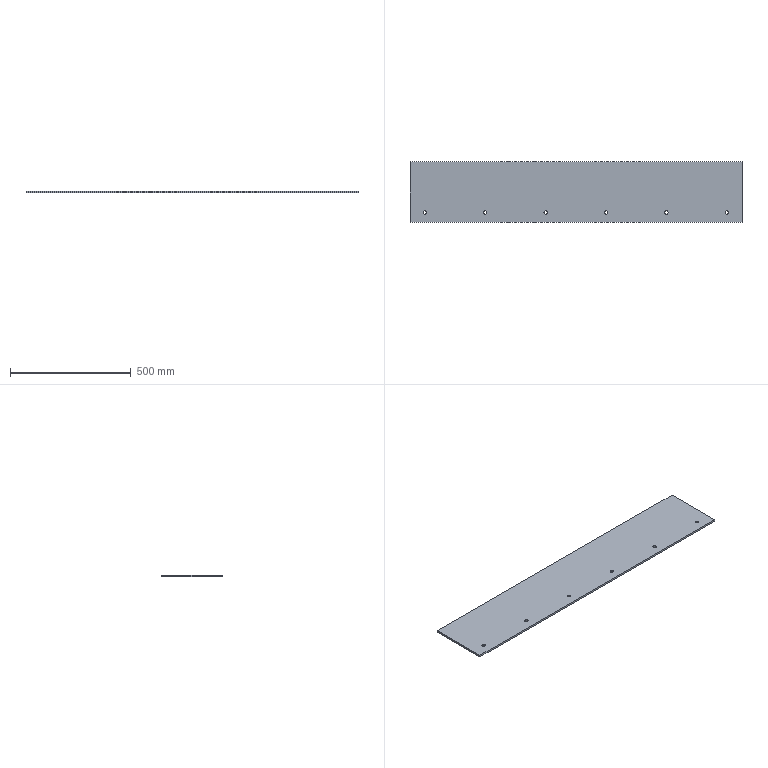Part | STEP file | Rubber plate 2_Default<As machined> | 1 solid | 18 faces | box 1374 x 250 x 8 mm | volume 2740611 mm3 | cylinder 12 | plane 6 | commonest cylinder face diameters 14 x12
STEP:
#1=CARTESIAN_POINT('',(0.,0.,0.));
#2=DIRECTION('',(0.,0.,1.));
#3=DIRECTION('',(1.,0.,0.));
#4=AXIS2_PLACEMENT_3D('',#1,#2,#3);
#5=CARTESIAN_POINT('',(-632.5,40.,8.));
#6=VERTEX_POINT('',#5);
#7=CARTESIAN_POINT('',(-632.5,40.,0.));
#8=VERTEX_POINT('',#7);
#9=CARTESIAN_POINT('',(-632.5,40.,8.));
#10=DIRECTION('',(0.,0.,-1.));
#11=VECTOR('',#10,1.);
#12=LINE('',#9,#11);
#13=CARTESIAN_POINT('',(-625.5,40.,8.));
#14=DIRECTION('',(0.,0.,-1.));
#15=DIRECTION('',(-1.,0.,0.));
#16=AXIS2_PLACEMENT_3D('',#13,#14,#15);
#17=CYLINDRICAL_SURFACE('',#16,7.);
#18=CARTESIAN_POINT('',(6.283,0.));
#19=DIRECTION('',(0.,1.));
#20=VECTOR('',#19,1.);
#21=LINE('',#18,#20);
#22=(GEOMETRIC_REPRESENTATION_CONTEXT(2)PARAMETRIC_REPRESENTATION_CONTEXT()REPRESENTATION_CONTEXT('',''));
#23=DEFINITIONAL_REPRESENTATION('',(#21),#22);
#24=PCURVE('',#17,#23);
#25=CARTESIAN_POINT('',(-625.5,40.,8.));
#26=DIRECTION('',(0.,0.,-1.));
#27=DIRECTION('',(-1.,0.,0.));
#28=AXIS2_PLACEMENT_3D('',#25,#26,#27);
#29=CYLINDRICAL_SURFACE('',#28,7.);
#30=CARTESIAN_POINT('',(0.,0.));
#31=DIRECTION('',(0.,1.));
#32=VECTOR('',#31,1.);
#33=LINE('',#30,#32);
#34=(GEOMETRIC_REPRESENTATION_CONTEXT(2)PARAMETRIC_REPRESENTATION_CONTEXT()REPRESENTATION_CONTEXT('',''));
#35=DEFINITIONAL_REPRESENTATION('',(#33),#34);
#36=PCURVE('',#29,#35);
#37=SURFACE_CURVE('',#12,(#24,#36),.PCURVE_S1.);
#38=EDGE_CURVE('',#6,#8,#37,.T.);
#39=ORIENTED_EDGE('',*,*,#38,.T.);
#40=CARTESIAN_POINT('',(-618.5,40.,0.));
#41=VERTEX_POINT('',#40);
#42=CARTESIAN_POINT('',(-625.5,40.,0.));
#43=DIRECTION('',(0.,0.,1.));
#44=DIRECTION('',(1.,0.,0.));
#45=AXIS2_PLACEMENT_3D('',#42,#43,#44);
#46=CIRCLE('',#45,7.);
#47=CARTESIAN_POINT('',(9.425,8.));
#48=DIRECTION('',(-1.,0.));
#49=VECTOR('',#48,1.);
#50=LINE('',#47,#49);
#51=(GEOMETRIC_REPRESENTATION_CONTEXT(2)PARAMETRIC_REPRESENTATION_CONTEXT()REPRESENTATION_CONTEXT('',''));
#52=DEFINITIONAL_REPRESENTATION('',(#50),#51);
#53=PCURVE('',#17,#52);
#54=CARTESIAN_POINT('',(0.,0.,0.));
#55=DIRECTION('',(0.,0.,1.));
#56=DIRECTION('',(1.,0.,0.));
#57=AXIS2_PLACEMENT_3D('',#54,#55,#56);
#58=PLANE('',#57);
#59=CARTESIAN_POINT('',(-625.5,40.));
#60=DIRECTION('',(1.,0.));
#61=AXIS2_PLACEMENT_2D('',#59,#60);
#62=CIRCLE('',#61,7.);
#63=(GEOMETRIC_REPRESENTATION_CONTEXT(2)PARAMETRIC_REPRESENTATION_CONTEXT()REPRESENTATION_CONTEXT('',''));
#64=DEFINITIONAL_REPRESENTATION('',(#62),#63);
#65=PCURVE('',#58,#64);
#66=SURFACE_CURVE('',#46,(#53,#65),.PCURVE_S1.);
#67=EDGE_CURVE('',#8,#41,#66,.T.);
#68=ORIENTED_EDGE('',*,*,#67,.T.);
#69=CARTESIAN_POINT('',(-618.5,40.,8.));
#70=VERTEX_POINT('',#69);
#71=CARTESIAN_POINT('',(-618.5,40.,8.));
#72=DIRECTION('',(0.,0.,-1.));
#73=VECTOR('',#72,1.);
#74=LINE('',#71,#73);
#75=CARTESIAN_POINT('',(3.142,0.));
#76=DIRECTION('',(0.,1.));
#77=VECTOR('',#76,1.);
#78=LINE('',#75,#77);
#79=(GEOMETRIC_REPRESENTATION_CONTEXT(2)PARAMETRIC_REPRESENTATION_CONTEXT()REPRESENTATION_CONTEXT('',''));
#80=DEFINITIONAL_REPRESENTATION('',(#78),#79);
#81=PCURVE('',#17,#80);
#82=CARTESIAN_POINT('',(3.142,0.));
#83=DIRECTION('',(0.,1.));
#84=VECTOR('',#83,1.);
#85=LINE('',#82,#84);
#86=(GEOMETRIC_REPRESENTATION_CONTEXT(2)PARAMETRIC_REPRESENTATION_CONTEXT()REPRESENTATION_CONTEXT('',''));
#87=DEFINITIONAL_REPRESENTATION('',(#85),#86);
#88=PCURVE('',#29,#87);
#89=SURFACE_CURVE('',#74,(#81,#88),.PCURVE_S1.);
#90=EDGE_CURVE('',#70,#41,#89,.T.);
#91=ORIENTED_EDGE('',*,*,#90,.F.);
#92=CARTESIAN_POINT('',(-625.5,40.,8.));
#93=DIRECTION('',(0.,0.,1.));
#94=DIRECTION('',(1.,0.,0.));
#95=AXIS2_PLACEMENT_3D('',#92,#93,#94);
#96=CIRCLE('',#95,7.);
#97=CARTESIAN_POINT('',(9.425,0.));
#98=DIRECTION('',(-1.,0.));
#99=VECTOR('',#98,1.);
#100=LINE('',#97,#99);
#101=(GEOMETRIC_REPRESENTATION_CONTEXT(2)PARAMETRIC_REPRESENTATION_CONTEXT()REPRESENTATION_CONTEXT('',''));
#102=DEFINITIONAL_REPRESENTATION('',(#100),#101);
#103=PCURVE('',#17,#102);
#104=CARTESIAN_POINT('',(0.,0.,8.));
#105=DIRECTION('',(0.,0.,1.));
#106=DIRECTION('',(1.,0.,0.));
#107=AXIS2_PLACEMENT_3D('',#104,#105,#106);
#108=PLANE('',#107);
#109=CARTESIAN_POINT('',(-625.5,40.));
#110=DIRECTION('',(1.,0.));
#111=AXIS2_PLACEMENT_2D('',#109,#110);
#112=CIRCLE('',#111,7.);
#113=(GEOMETRIC_REPRESENTATION_CONTEXT(2)PARAMETRIC_REPRESENTATION_CONTEXT()REPRESENTATION_CONTEXT('',''));
#114=DEFINITIONAL_REPRESENTATION('',(#112),#113);
#115=PCURVE('',#108,#114);
#116=SURFACE_CURVE('',#96,(#103,#115),.PCURVE_S1.);
#117=EDGE_CURVE('',#6,#70,#116,.T.);
#118=ORIENTED_EDGE('',*,*,#117,.F.);
#119=EDGE_LOOP('',(#39,#68,#91,#118));
#120=FACE_BOUND('',#119,.F.);
#121=ADVANCED_FACE('',(#120),#17,.F.);
#122=CARTESIAN_POINT('',(-382.5,40.,8.));
#123=VERTEX_POINT('',#122);
#124=CARTESIAN_POINT('',(-382.5,40.,0.));
#125=VERTEX_POINT('',#124);
#126=CARTESIAN_POINT('',(-382.5,40.,8.));
#127=DIRECTION('',(0.,0.,-1.));
#128=VECTOR('',#127,1.);
#129=LINE('',#126,#128);
#130=CARTESIAN_POINT('',(-375.5,40.,8.));
#131=DIRECTION('',(0.,0.,-1.));
#132=DIRECTION('',(-1.,0.,0.));
#133=AXIS2_PLACEMENT_3D('',#130,#131,#132);
#134=CYLINDRICAL_SURFACE('',#133,7.);
#135=CARTESIAN_POINT('',(6.283,0.));
#136=DIRECTION('',(0.,1.));
#137=VECTOR('',#136,1.);
#138=LINE('',#135,#137);
#139=(GEOMETRIC_REPRESENTATION_CONTEXT(2)PARAMETRIC_REPRESENTATION_CONTEXT()REPRESENTATION_CONTEXT('',''));
#140=DEFINITIONAL_REPRESENTATION('',(#138),#139);
#141=PCURVE('',#134,#140);
#142=CARTESIAN_POINT('',(-375.5,40.,8.));
#143=DIRECTION('',(0.,0.,-1.));
#144=DIRECTION('',(-1.,0.,0.));
#145=AXIS2_PLACEMENT_3D('',#142,#143,#144);
#146=CYLINDRICAL_SURFACE('',#145,7.);
#147=CARTESIAN_POINT('',(0.,0.));
#148=DIRECTION('',(0.,1.));
#149=VECTOR('',#148,1.);
#150=LINE('',#147,#149);
#151=(GEOMETRIC_REPRESENTATION_CONTEXT(2)PARAMETRIC_REPRESENTATION_CONTEXT()REPRESENTATION_CONTEXT('',''));
#152=DEFINITIONAL_REPRESENTATION('',(#150),#151);
#153=PCURVE('',#146,#152);
#154=SURFACE_CURVE('',#129,(#141,#153),.PCURVE_S1.);
#155=EDGE_CURVE('',#123,#125,#154,.T.);
#156=ORIENTED_EDGE('',*,*,#155,.T.);
#157=CARTESIAN_POINT('',(-368.5,40.,0.));
#158=VERTEX_POINT('',#157);
#159=CARTESIAN_POINT('',(-375.5,40.,0.));
#160=DIRECTION('',(0.,0.,1.));
#161=DIRECTION('',(1.,0.,0.));
#162=AXIS2_PLACEMENT_3D('',#159,#160,#161);
#163=CIRCLE('',#162,7.);
#164=CARTESIAN_POINT('',(9.425,8.));
#165=DIRECTION('',(-1.,0.));
#166=VECTOR('',#165,1.);
#167=LINE('',#164,#166);
#168=(GEOMETRIC_REPRESENTATION_CONTEXT(2)PARAMETRIC_REPRESENTATION_CONTEXT()REPRESENTATION_CONTEXT('',''));
#169=DEFINITIONAL_REPRESENTATION('',(#167),#168);
#170=PCURVE('',#134,#169);
#171=CARTESIAN_POINT('',(-375.5,40.));
#172=DIRECTION('',(1.,0.));
#173=AXIS2_PLACEMENT_2D('',#171,#172);
#174=CIRCLE('',#173,7.);
#175=(GEOMETRIC_REPRESENTATION_CONTEXT(2)PARAMETRIC_REPRESENTATION_CONTEXT()REPRESENTATION_CONTEXT('',''));
#176=DEFINITIONAL_REPRESENTATION('',(#174),#175);
#177=PCURVE('',#58,#176);
#178=SURFACE_CURVE('',#163,(#170,#177),.PCURVE_S1.);
#179=EDGE_CURVE('',#125,#158,#178,.T.);
#180=ORIENTED_EDGE('',*,*,#179,.T.);
#181=CARTESIAN_POINT('',(-368.5,40.,8.));
#182=VERTEX_POINT('',#181);
#183=CARTESIAN_POINT('',(-368.5,40.,8.));
#184=DIRECTION('',(0.,0.,-1.));
#185=VECTOR('',#184,1.);
#186=LINE('',#183,#185);
#187=CARTESIAN_POINT('',(3.142,0.));
#188=DIRECTION('',(0.,1.));
#189=VECTOR('',#188,1.);
#190=LINE('',#187,#189);
#191=(GEOMETRIC_REPRESENTATION_CONTEXT(2)PARAMETRIC_REPRESENTATION_CONTEXT()REPRESENTATION_CONTEXT('',''));
#192=DEFINITIONAL_REPRESENTATION('',(#190),#191);
#193=PCURVE('',#134,#192);
#194=CARTESIAN_POINT('',(3.142,0.));
#195=DIRECTION('',(0.,1.));
#196=VECTOR('',#195,1.);
#197=LINE('',#194,#196);
#198=(GEOMETRIC_REPRESENTATION_CONTEXT(2)PARAMETRIC_REPRESENTATION_CONTEXT()REPRESENTATION_CONTEXT('',''));
#199=DEFINITIONAL_REPRESENTATION('',(#197),#198);
#200=PCURVE('',#146,#199);
#201=SURFACE_CURVE('',#186,(#193,#200),.PCURVE_S1.);
#202=EDGE_CURVE('',#182,#158,#201,.T.);
#203=ORIENTED_EDGE('',*,*,#202,.F.);
#204=CARTESIAN_POINT('',(-375.5,40.,8.));
#205=DIRECTION('',(0.,0.,1.));
#206=DIRECTION('',(1.,0.,0.));
#207=AXIS2_PLACEMENT_3D('',#204,#205,#206);
#208=CIRCLE('',#207,7.);
#209=CARTESIAN_POINT('',(9.425,0.));
#210=DIRECTION('',(-1.,0.));
#211=VECTOR('',#210,1.);
#212=LINE('',#209,#211);
#213=(GEOMETRIC_REPRESENTATION_CONTEXT(2)PARAMETRIC_REPRESENTATION_CONTEXT()REPRESENTATION_CONTEXT('',''));
#214=DEFINITIONAL_REPRESENTATION('',(#212),#213);
#215=PCURVE('',#134,#214);
#216=CARTESIAN_POINT('',(-375.5,40.));
#217=DIRECTION('',(1.,0.));
#218=AXIS2_PLACEMENT_2D('',#216,#217);
#219=CIRCLE('',#218,7.);
#220=(GEOMETRIC_REPRESENTATION_CONTEXT(2)PARAMETRIC_REPRESENTATION_CONTEXT()REPRESENTATION_CONTEXT('',''));
#221=DEFINITIONAL_REPRESENTATION('',(#219),#220);
#222=PCURVE('',#108,#221);
#223=SURFACE_CURVE('',#208,(#215,#222),.PCURVE_S1.);
#224=EDGE_CURVE('',#123,#182,#223,.T.);
#225=ORIENTED_EDGE('',*,*,#224,.F.);
#226=EDGE_LOOP('',(#156,#180,#203,#225));
#227=FACE_BOUND('',#226,.F.);
#228=ADVANCED_FACE('',(#227),#134,.F.);
#229=CARTESIAN_POINT('',(-132.5,40.,8.));
#230=VERTEX_POINT('',#229);
#231=CARTESIAN_POINT('',(-132.5,40.,0.));
#232=VERTEX_POINT('',#231);
#233=CARTESIAN_POINT('',(-132.5,40.,8.));
#234=DIRECTION('',(0.,0.,-1.));
#235=VECTOR('',#234,1.);
#236=LINE('',#233,#235);
#237=CARTESIAN_POINT('',(-125.5,40.,8.));
#238=DIRECTION('',(0.,0.,-1.));
#239=DIRECTION('',(-1.,0.,0.));
#240=AXIS2_PLACEMENT_3D('',#237,#238,#239);
#241=CYLINDRICAL_SURFACE('',#240,7.);
#242=CARTESIAN_POINT('',(6.283,0.));
#243=DIRECTION('',(0.,1.));
#244=VECTOR('',#243,1.);
#245=LINE('',#242,#244);
#246=(GEOMETRIC_REPRESENTATION_CONTEXT(2)PARAMETRIC_REPRESENTATION_CONTEXT()REPRESENTATION_CONTEXT('',''));
#247=DEFINITIONAL_REPRESENTATION('',(#245),#246);
#248=PCURVE('',#241,#247);
#249=CARTESIAN_POINT('',(-125.5,40.,8.));
#250=DIRECTION('',(0.,0.,-1.));
#251=DIRECTION('',(-1.,0.,0.));
#252=AXIS2_PLACEMENT_3D('',#249,#250,#251);
#253=CYLINDRICAL_SURFACE('',#252,7.);
#254=CARTESIAN_POINT('',(0.,0.));
#255=DIRECTION('',(0.,1.));
#256=VECTOR('',#255,1.);
#257=LINE('',#254,#256);
#258=(GEOMETRIC_REPRESENTATION_CONTEXT(2)PARAMETRIC_REPRESENTATION_CONTEXT()REPRESENTATION_CONTEXT('',''));
#259=DEFINITIONAL_REPRESENTATION('',(#257),#258);
#260=PCURVE('',#253,#259);
#261=SURFACE_CURVE('',#236,(#248,#260),.PCURVE_S1.);
#262=EDGE_CURVE('',#230,#232,#261,.T.);
#263=ORIENTED_EDGE('',*,*,#262,.T.);
#264=CARTESIAN_POINT('',(-118.5,40.,0.));
#265=VERTEX_POINT('',#264);
#266=CARTESIAN_POINT('',(-125.5,40.,0.));
#267=DIRECTION('',(0.,0.,1.));
#268=DIRECTION('',(1.,0.,0.));
#269=AXIS2_PLACEMENT_3D('',#266,#267,#268);
#270=CIRCLE('',#269,7.);
#271=CARTESIAN_POINT('',(9.425,8.));
#272=DIRECTION('',(-1.,0.));
#273=VECTOR('',#272,1.);
#274=LINE('',#271,#273);
#275=(GEOMETRIC_REPRESENTATION_CONTEXT(2)PARAMETRIC_REPRESENTATION_CONTEXT()REPRESENTATION_CONTEXT('',''));
#276=DEFINITIONAL_REPRESENTATION('',(#274),#275);
#277=PCURVE('',#241,#276);
#278=CARTESIAN_POINT('',(-125.5,40.));
#279=DIRECTION('',(1.,0.));
#280=AXIS2_PLACEMENT_2D('',#278,#279);
#281=CIRCLE('',#280,7.);
#282=(GEOMETRIC_REPRESENTATION_CONTEXT(2)PARAMETRIC_REPRESENTATION_CONTEXT()REPRESENTATION_CONTEXT('',''));
#283=DEFINITIONAL_REPRESENTATION('',(#281),#282);
#284=PCURVE('',#58,#283);
#285=SURFACE_CURVE('',#270,(#277,#284),.PCURVE_S1.);
#286=EDGE_CURVE('',#232,#265,#285,.T.);
#287=ORIENTED_EDGE('',*,*,#286,.T.);
#288=CARTESIAN_POINT('',(-118.5,40.,8.));
#289=VERTEX_POINT('',#288);
#290=CARTESIAN_POINT('',(-118.5,40.,8.));
#291=DIRECTION('',(0.,0.,-1.));
#292=VECTOR('',#291,1.);
#293=LINE('',#290,#292);
#294=CARTESIAN_POINT('',(3.142,0.));
#295=DIRECTION('',(0.,1.));
#296=VECTOR('',#295,1.);
#297=LINE('',#294,#296);
#298=(GEOMETRIC_REPRESENTATION_CONTEXT(2)PARAMETRIC_REPRESENTATION_CONTEXT()REPRESENTATION_CONTEXT('',''));
#299=DEFINITIONAL_REPRESENTATION('',(#297),#298);
#300=PCURVE('',#241,#299);
#301=CARTESIAN_POINT('',(3.142,0.));
#302=DIRECTION('',(0.,1.));
#303=VECTOR('',#302,1.);
#304=LINE('',#301,#303);
#305=(GEOMETRIC_REPRESENTATION_CONTEXT(2)PARAMETRIC_REPRESENTATION_CONTEXT()REPRESENTATION_CONTEXT('',''));
#306=DEFINITIONAL_REPRESENTATION('',(#304),#305);
#307=PCURVE('',#253,#306);
#308=SURFACE_CURVE('',#293,(#300,#307),.PCURVE_S1.);
#309=EDGE_CURVE('',#289,#265,#308,.T.);
#310=ORIENTED_EDGE('',*,*,#309,.F.);
#311=CARTESIAN_POINT('',(-125.5,40.,8.));
#312=DIRECTION('',(0.,0.,1.));
#313=DIRECTION('',(1.,0.,0.));
#314=AXIS2_PLACEMENT_3D('',#311,#312,#313);
#315=CIRCLE('',#314,7.);
#316=CARTESIAN_POINT('',(9.425,0.));
#317=DIRECTION('',(-1.,0.));
#318=VECTOR('',#317,1.);
#319=LINE('',#316,#318);
#320=(GEOMETRIC_REPRESENTATION_CONTEXT(2)PARAMETRIC_REPRESENTATION_CONTEXT()REPRESENTATION_CONTEXT('',''));
#321=DEFINITIONAL_REPRESENTATION('',(#319),#320);
#322=PCURVE('',#241,#321);
#323=CARTESIAN_POINT('',(-125.5,40.));
#324=DIRECTION('',(1.,0.));
#325=AXIS2_PLACEMENT_2D('',#323,#324);
#326=CIRCLE('',#325,7.);
#327=(GEOMETRIC_REPRESENTATION_CONTEXT(2)PARAMETRIC_REPRESENTATION_CONTEXT()REPRESENTATION_CONTEXT('',''));
#328=DEFINITIONAL_REPRESENTATION('',(#326),#327);
#329=PCURVE('',#108,#328);
#330=SURFACE_CURVE('',#315,(#322,#329),.PCURVE_S1.);
#331=EDGE_CURVE('',#230,#289,#330,.T.);
#332=ORIENTED_EDGE('',*,*,#331,.F.);
#333=EDGE_LOOP('',(#263,#287,#310,#332));
#334=FACE_BOUND('',#333,.F.);
#335=ADVANCED_FACE('',(#334),#241,.F.);
#336=CARTESIAN_POINT('',(117.5,40.,8.));
#337=VERTEX_POINT('',#336);
#338=CARTESIAN_POINT('',(117.5,40.,0.));
#339=VERTEX_POINT('',#338);
#340=CARTESIAN_POINT('',(117.5,40.,8.));
#341=DIRECTION('',(0.,0.,-1.));
#342=VECTOR('',#341,1.);
#343=LINE('',#340,#342);
#344=CARTESIAN_POINT('',(124.5,40.,8.));
#345=DIRECTION('',(0.,0.,-1.));
#346=DIRECTION('',(-1.,0.,0.));
#347=AXIS2_PLACEMENT_3D('',#344,#345,#346);
#348=CYLINDRICAL_SURFACE('',#347,7.);
#349=CARTESIAN_POINT('',(6.283,0.));
#350=DIRECTION('',(0.,1.));
#351=VECTOR('',#350,1.);
#352=LINE('',#349,#351);
#353=(GEOMETRIC_REPRESENTATION_CONTEXT(2)PARAMETRIC_REPRESENTATION_CONTEXT()REPRESENTATION_CONTEXT('',''));
#354=DEFINITIONAL_REPRESENTATION('',(#352),#353);
#355=PCURVE('',#348,#354);
#356=CARTESIAN_POINT('',(124.5,40.,8.));
#357=DIRECTION('',(0.,0.,-1.));
#358=DIRECTION('',(-1.,0.,0.));
#359=AXIS2_PLACEMENT_3D('',#356,#357,#358);
#360=CYLINDRICAL_SURFACE('',#359,7.);
#361=CARTESIAN_POINT('',(0.,0.));
#362=DIRECTION('',(0.,1.));
#363=VECTOR('',#362,1.);
#364=LINE('',#361,#363);
#365=(GEOMETRIC_REPRESENTATION_CONTEXT(2)PARAMETRIC_REPRESENTATION_CONTEXT()REPRESENTATION_CONTEXT('',''));
#366=DEFINITIONAL_REPRESENTATION('',(#364),#365);
#367=PCURVE('',#360,#366);
#368=SURFACE_CURVE('',#343,(#355,#367),.PCURVE_S1.);
#369=EDGE_CURVE('',#337,#339,#368,.T.);
#370=ORIENTED_EDGE('',*,*,#369,.T.);
#371=CARTESIAN_POINT('',(131.5,40.,0.));
#372=VERTEX_POINT('',#371);
#373=CARTESIAN_POINT('',(124.5,40.,0.));
#374=DIRECTION('',(0.,0.,1.));
#375=DIRECTION('',(1.,0.,0.));
#376=AXIS2_PLACEMENT_3D('',#373,#374,#375);
#377=CIRCLE('',#376,7.);
#378=CARTESIAN_POINT('',(9.425,8.));
#379=DIRECTION('',(-1.,0.));
#380=VECTOR('',#379,1.);
#381=LINE('',#378,#380);
#382=(GEOMETRIC_REPRESENTATION_CONTEXT(2)PARAMETRIC_REPRESENTATION_CONTEXT()REPRESENTATION_CONTEXT('',''));
#383=DEFINITIONAL_REPRESENTATION('',(#381),#382);
#384=PCURVE('',#348,#383);
#385=CARTESIAN_POINT('',(124.5,40.));
#386=DIRECTION('',(1.,0.));
#387=AXIS2_PLACEMENT_2D('',#385,#386);
#388=CIRCLE('',#387,7.);
#389=(GEOMETRIC_REPRESENTATION_CONTEXT(2)PARAMETRIC_REPRESENTATION_CONTEXT()REPRESENTATION_CONTEXT('',''));
#390=DEFINITIONAL_REPRESENTATION('',(#388),#389);
#391=PCURVE('',#58,#390);
#392=SURFACE_CURVE('',#377,(#384,#391),.PCURVE_S1.);
#393=EDGE_CURVE('',#339,#372,#392,.T.);
#394=ORIENTED_EDGE('',*,*,#393,.T.);
#395=CARTESIAN_POINT('',(131.5,40.,8.));
#396=VERTEX_POINT('',#395);
#397=CARTESIAN_POINT('',(131.5,40.,8.));
#398=DIRECTION('',(0.,0.,-1.));
#399=VECTOR('',#398,1.);
#400=LINE('',#397,#399);
#401=CARTESIAN_POINT('',(3.142,0.));
#402=DIRECTION('',(0.,1.));
#403=VECTOR('',#402,1.);
#404=LINE('',#401,#403);
#405=(GEOMETRIC_REPRESENTATION_CONTEXT(2)PARAMETRIC_REPRESENTATION_CONTEXT()REPRESENTATION_CONTEXT('',''));
#406=DEFINITIONAL_REPRESENTATION('',(#404),#405);
#407=PCURVE('',#348,#406);
#408=CARTESIAN_POINT('',(3.142,0.));
#409=DIRECTION('',(0.,1.));
#410=VECTOR('',#409,1.);
#411=LINE('',#408,#410);
#412=(GEOMETRIC_REPRESENTATION_CONTEXT(2)PARAMETRIC_REPRESENTATION_CONTEXT()REPRESENTATION_CONTEXT('',''));
#413=DEFINITIONAL_REPRESENTATION('',(#411),#412);
#414=PCURVE('',#360,#413);
#415=SURFACE_CURVE('',#400,(#407,#414),.PCURVE_S1.);
#416=EDGE_CURVE('',#396,#372,#415,.T.);
#417=ORIENTED_EDGE('',*,*,#416,.F.);
#418=CARTESIAN_POINT('',(124.5,40.,8.));
#419=DIRECTION('',(0.,0.,1.));
#420=DIRECTION('',(1.,0.,0.));
#421=AXIS2_PLACEMENT_3D('',#418,#419,#420);
#422=CIRCLE('',#421,7.);
#423=CARTESIAN_POINT('',(9.425,0.));
#424=DIRECTION('',(-1.,0.));
#425=VECTOR('',#424,1.);
#426=LINE('',#423,#425);
#427=(GEOMETRIC_REPRESENTATION_CONTEXT(2)PARAMETRIC_REPRESENTATION_CONTEXT()REPRESENTATION_CONTEXT('',''));
#428=DEFINITIONAL_REPRESENTATION('',(#426),#427);
#429=PCURVE('',#348,#428);
#430=CARTESIAN_POINT('',(124.5,40.));
#431=DIRECTION('',(1.,0.));
#432=AXIS2_PLACEMENT_2D('',#430,#431);
#433=CIRCLE('',#432,7.);
#434=(GEOMETRIC_REPRESENTATION_CONTEXT(2)PARAMETRIC_REPRESENTATION_CONTEXT()REPRESENTATION_CONTEXT('',''));
#435=DEFINITIONAL_REPRESENTATION('',(#433),#434);
#436=PCURVE('',#108,#435);
#437=SURFACE_CURVE('',#422,(#429,#436),.PCURVE_S1.);
#438=EDGE_CURVE('',#337,#396,#437,.T.);
#439=ORIENTED_EDGE('',*,*,#438,.F.);
#440=EDGE_LOOP('',(#370,#394,#417,#439));
#441=FACE_BOUND('',#440,.F.);
#442=ADVANCED_FACE('',(#441),#348,.F.);
#443=CARTESIAN_POINT('',(367.5,40.,8.));
#444=VERTEX_POINT('',#443);
#445=CARTESIAN_POINT('',(367.5,40.,0.));
#446=VERTEX_POINT('',#445);
#447=CARTESIAN_POINT('',(367.5,40.,8.));
#448=DIRECTION('',(0.,0.,-1.));
#449=VECTOR('',#448,1.);
#450=LINE('',#447,#449);
#451=CARTESIAN_POINT('',(374.5,40.,8.));
#452=DIRECTION('',(0.,0.,-1.));
#453=DIRECTION('',(-1.,0.,0.));
#454=AXIS2_PLACEMENT_3D('',#451,#452,#453);
#455=CYLINDRICAL_SURFACE('',#454,7.);
#456=CARTESIAN_POINT('',(6.283,0.));
#457=DIRECTION('',(0.,1.));
#458=VECTOR('',#457,1.);
#459=LINE('',#456,#458);
#460=(GEOMETRIC_REPRESENTATION_CONTEXT(2)PARAMETRIC_REPRESENTATION_CONTEXT()REPRESENTATION_CONTEXT('',''));
#461=DEFINITIONAL_REPRESENTATION('',(#459),#460);
#462=PCURVE('',#455,#461);
#463=CARTESIAN_POINT('',(374.5,40.,8.));
#464=DIRECTION('',(0.,0.,-1.));
#465=DIRECTION('',(-1.,0.,0.));
#466=AXIS2_PLACEMENT_3D('',#463,#464,#465);
#467=CYLINDRICAL_SURFACE('',#466,7.);
#468=CARTESIAN_POINT('',(0.,0.));
#469=DIRECTION('',(0.,1.));
#470=VECTOR('',#469,1.);
#471=LINE('',#468,#470);
#472=(GEOMETRIC_REPRESENTATION_CONTEXT(2)PARAMETRIC_REPRESENTATION_CONTEXT()REPRESENTATION_CONTEXT('',''));
#473=DEFINITIONAL_REPRESENTATION('',(#471),#472);
#474=PCURVE('',#467,#473);
#475=SURFACE_CURVE('',#450,(#462,#474),.PCURVE_S1.);
#476=EDGE_CURVE('',#444,#446,#475,.T.);
#477=ORIENTED_EDGE('',*,*,#476,.T.);
#478=CARTESIAN_POINT('',(381.5,40.,0.));
#479=VERTEX_POINT('',#478);
#480=CARTESIAN_POINT('',(374.5,40.,0.));
#481=DIRECTION('',(0.,0.,1.));
#482=DIRECTION('',(1.,0.,0.));
#483=AXIS2_PLACEMENT_3D('',#480,#481,#482);
#484=CIRCLE('',#483,7.);
#485=CARTESIAN_POINT('',(9.425,8.));
#486=DIRECTION('',(-1.,0.));
#487=VECTOR('',#486,1.);
#488=LINE('',#485,#487);
#489=(GEOMETRIC_REPRESENTATION_CONTEXT(2)PARAMETRIC_REPRESENTATION_CONTEXT()REPRESENTATION_CONTEXT('',''));
#490=DEFINITIONAL_REPRESENTATION('',(#488),#489);
#491=PCURVE('',#455,#490);
#492=CARTESIAN_POINT('',(374.5,40.));
#493=DIRECTION('',(1.,0.));
#494=AXIS2_PLACEMENT_2D('',#492,#493);
#495=CIRCLE('',#494,7.);
#496=(GEOMETRIC_REPRESENTATION_CONTEXT(2)PARAMETRIC_REPRESENTATION_CONTEXT()REPRESENTATION_CONTEXT('',''));
#497=DEFINITIONAL_REPRESENTATION('',(#495),#496);
#498=PCURVE('',#58,#497);
#499=SURFACE_CURVE('',#484,(#491,#498),.PCURVE_S1.);
#500=EDGE_CURVE('',#446,#479,#499,.T.);
#501=ORIENTED_EDGE('',*,*,#500,.T.);
#502=CARTESIAN_POINT('',(381.5,40.,8.));
#503=VERTEX_POINT('',#502);
#504=CARTESIAN_POINT('',(381.5,40.,8.));
#505=DIRECTION('',(0.,0.,-1.));
#506=VECTOR('',#505,1.);
#507=LINE('',#504,#506);
#508=CARTESIAN_POINT('',(3.142,0.));
#509=DIRECTION('',(0.,1.));
#510=VECTOR('',#509,1.);
#511=LINE('',#508,#510);
#512=(GEOMETRIC_REPRESENTATION_CONTEXT(2)PARAMETRIC_REPRESENTATION_CONTEXT()REPRESENTATION_CONTEXT('',''));
#513=DEFINITIONAL_REPRESENTATION('',(#511),#512);
#514=PCURVE('',#455,#513);
#515=CARTESIAN_POINT('',(3.142,0.));
#516=DIRECTION('',(0.,1.));
#517=VECTOR('',#516,1.);
#518=LINE('',#515,#517);
#519=(GEOMETRIC_REPRESENTATION_CONTEXT(2)PARAMETRIC_REPRESENTATION_CONTEXT()REPRESENTATION_CONTEXT('',''));
#520=DEFINITIONAL_REPRESENTATION('',(#518),#519);
#521=PCURVE('',#467,#520);
#522=SURFACE_CURVE('',#507,(#514,#521),.PCURVE_S1.);
#523=EDGE_CURVE('',#503,#479,#522,.T.);
#524=ORIENTED_EDGE('',*,*,#523,.F.);
#525=CARTESIAN_POINT('',(374.5,40.,8.));
#526=DIRECTION('',(0.,0.,1.));
#527=DIRECTION('',(1.,0.,0.));
#528=AXIS2_PLACEMENT_3D('',#525,#526,#527);
#529=CIRCLE('',#528,7.);
#530=CARTESIAN_POINT('',(9.425,0.));
#531=DIRECTION('',(-1.,0.));
#532=VECTOR('',#531,1.);
#533=LINE('',#530,#532);
#534=(GEOMETRIC_REPRESENTATION_CONTEXT(2)PARAMETRIC_REPRESENTATION_CONTEXT()REPRESENTATION_CONTEXT('',''));
#535=DEFINITIONAL_REPRESENTATION('',(#533),#534);
#536=PCURVE('',#455,#535);
#537=CARTESIAN_POINT('',(374.5,40.));
#538=DIRECTION('',(1.,0.));
#539=AXIS2_PLACEMENT_2D('',#537,#538);
#540=CIRCLE('',#539,7.);
#541=(GEOMETRIC_REPRESENTATION_CONTEXT(2)PARAMETRIC_REPRESENTATION_CONTEXT()REPRESENTATION_CONTEXT('',''));
#542=DEFINITIONAL_REPRESENTATION('',(#540),#541);
#543=PCURVE('',#108,#542);
#544=SURFACE_CURVE('',#529,(#536,#543),.PCURVE_S1.);
#545=EDGE_CURVE('',#444,#503,#544,.T.);
#546=ORIENTED_EDGE('',*,*,#545,.F.);
#547=EDGE_LOOP('',(#477,#501,#524,#546));
#548=FACE_BOUND('',#547,.F.);
#549=ADVANCED_FACE('',(#548),#455,.F.);
#550=CARTESIAN_POINT('',(617.5,40.,8.));
#551=VERTEX_POINT('',#550);
#552=CARTESIAN_POINT('',(617.5,40.,0.));
#553=VERTEX_POINT('',#552);
#554=CARTESIAN_POINT('',(617.5,40.,8.));
#555=DIRECTION('',(0.,0.,-1.));
#556=VECTOR('',#555,1.);
#557=LINE('',#554,#556);
#558=CARTESIAN_POINT('',(624.5,40.,8.));
#559=DIRECTION('',(0.,0.,-1.));
#560=DIRECTION('',(-1.,0.,0.));
#561=AXIS2_PLACEMENT_3D('',#558,#559,#560);
#562=CYLINDRICAL_SURFACE('',#561,7.);
#563=CARTESIAN_POINT('',(6.283,0.));
#564=DIRECTION('',(0.,1.));
#565=VECTOR('',#564,1.);
#566=LINE('',#563,#565);
#567=(GEOMETRIC_REPRESENTATION_CONTEXT(2)PARAMETRIC_REPRESENTATION_CONTEXT()REPRESENTATION_CONTEXT('',''));
#568=DEFINITIONAL_REPRESENTATION('',(#566),#567);
#569=PCURVE('',#562,#568);
#570=CARTESIAN_POINT('',(624.5,40.,8.));
#571=DIRECTION('',(0.,0.,-1.));
#572=DIRECTION('',(-1.,0.,0.));
#573=AXIS2_PLACEMENT_3D('',#570,#571,#572);
#574=CYLINDRICAL_SURFACE('',#573,7.);
#575=CARTESIAN_POINT('',(0.,0.));
#576=DIRECTION('',(0.,1.));
#577=VECTOR('',#576,1.);
#578=LINE('',#575,#577);
#579=(GEOMETRIC_REPRESENTATION_CONTEXT(2)PARAMETRIC_REPRESENTATION_CONTEXT()REPRESENTATION_CONTEXT('',''));
#580=DEFINITIONAL_REPRESENTATION('',(#578),#579);
#581=PCURVE('',#574,#580);
#582=SURFACE_CURVE('',#557,(#569,#581),.PCURVE_S1.);
#583=EDGE_CURVE('',#551,#553,#582,.T.);
#584=ORIENTED_EDGE('',*,*,#583,.T.);
#585=CARTESIAN_POINT('',(631.5,40.,0.));
#586=VERTEX_POINT('',#585);
#587=CARTESIAN_POINT('',(624.5,40.,0.));
#588=DIRECTION('',(0.,0.,1.));
#589=DIRECTION('',(1.,0.,0.));
#590=AXIS2_PLACEMENT_3D('',#587,#588,#589);
#591=CIRCLE('',#590,7.);
#592=CARTESIAN_POINT('',(9.425,8.));
#593=DIRECTION('',(-1.,0.));
#594=VECTOR('',#593,1.);
#595=LINE('',#592,#594);
#596=(GEOMETRIC_REPRESENTATION_CONTEXT(2)PARAMETRIC_REPRESENTATION_CONTEXT()REPRESENTATION_CONTEXT('',''));
#597=DEFINITIONAL_REPRESENTATION('',(#595),#596);
#598=PCURVE('',#562,#597);
#599=CARTESIAN_POINT('',(624.5,40.));
#600=DIRECTION('',(1.,0.));
#601=AXIS2_PLACEMENT_2D('',#599,#600);
#602=CIRCLE('',#601,7.);
#603=(GEOMETRIC_REPRESENTATION_CONTEXT(2)PARAMETRIC_REPRESENTATION_CONTEXT()REPRESENTATION_CONTEXT('',''));
#604=DEFINITIONAL_REPRESENTATION('',(#602),#603);
#605=PCURVE('',#58,#604);
#606=SURFACE_CURVE('',#591,(#598,#605),.PCURVE_S1.);
#607=EDGE_CURVE('',#553,#586,#606,.T.);
#608=ORIENTED_EDGE('',*,*,#607,.T.);
#609=CARTESIAN_POINT('',(631.5,40.,8.));
#610=VERTEX_POINT('',#609);
#611=CARTESIAN_POINT('',(631.5,40.,8.));
#612=DIRECTION('',(0.,0.,-1.));
#613=VECTOR('',#612,1.);
#614=LINE('',#611,#613);
#615=CARTESIAN_POINT('',(3.142,0.));
#616=DIRECTION('',(0.,1.));
#617=VECTOR('',#616,1.);
#618=LINE('',#615,#617);
#619=(GEOMETRIC_REPRESENTATION_CONTEXT(2)PARAMETRIC_REPRESENTATION_CONTEXT()REPRESENTATION_CONTEXT('',''));
#620=DEFINITIONAL_REPRESENTATION('',(#618),#619);
#621=PCURVE('',#562,#620);
#622=CARTESIAN_POINT('',(3.142,0.));
#623=DIRECTION('',(0.,1.));
#624=VECTOR('',#623,1.);
#625=LINE('',#622,#624);
#626=(GEOMETRIC_REPRESENTATION_CONTEXT(2)PARAMETRIC_REPRESENTATION_CONTEXT()REPRESENTATION_CONTEXT('',''));
#627=DEFINITIONAL_REPRESENTATION('',(#625),#626);
#628=PCURVE('',#574,#627);
#629=SURFACE_CURVE('',#614,(#621,#628),.PCURVE_S1.);
#630=EDGE_CURVE('',#610,#586,#629,.T.);
#631=ORIENTED_EDGE('',*,*,#630,.F.);
#632=CARTESIAN_POINT('',(624.5,40.,8.));
#633=DIRECTION('',(0.,0.,1.));
#634=DIRECTION('',(1.,0.,0.));
#635=AXIS2_PLACEMENT_3D('',#632,#633,#634);
#636=CIRCLE('',#635,7.);
#637=CARTESIAN_POINT('',(9.425,0.));
#638=DIRECTION('',(-1.,0.));
#639=VECTOR('',#638,1.);
#640=LINE('',#637,#639);
#641=(GEOMETRIC_REPRESENTATION_CONTEXT(2)PARAMETRIC_REPRESENTATION_CONTEXT()REPRESENTATION_CONTEXT('',''));
#642=DEFINITIONAL_REPRESENTATION('',(#640),#641);
#643=PCURVE('',#562,#642);
#644=CARTESIAN_POINT('',(624.5,40.));
#645=DIRECTION('',(1.,0.));
#646=AXIS2_PLACEMENT_2D('',#644,#645);
#647=CIRCLE('',#646,7.);
#648=(GEOMETRIC_REPRESENTATION_CONTEXT(2)PARAMETRIC_REPRESENTATION_CONTEXT()REPRESENTATION_CONTEXT('',''));
#649=DEFINITIONAL_REPRESENTATION('',(#647),#648);
#650=PCURVE('',#108,#649);
#651=SURFACE_CURVE('',#636,(#643,#650),.PCURVE_S1.);
#652=EDGE_CURVE('',#551,#610,#651,.T.);
#653=ORIENTED_EDGE('',*,*,#652,.F.);
#654=EDGE_LOOP('',(#584,#608,#631,#653));
#655=FACE_BOUND('',#654,.F.);
#656=ADVANCED_FACE('',(#655),#562,.F.);
#657=CARTESIAN_POINT('',(-687.,250.,0.));
#658=VERTEX_POINT('',#657);
#659=CARTESIAN_POINT('',(687.,250.,0.));
#660=VERTEX_POINT('',#659);
#661=CARTESIAN_POINT('',(0.,250.,0.));
#662=DIRECTION('',(1.,0.,0.));
#663=VECTOR('',#662,1.);
#664=LINE('',#661,#663);
#665=CARTESIAN_POINT('',(0.,250.,8.));
#666=DIRECTION('',(0.,1.,0.));
#667=DIRECTION('',(0.,0.,1.));
#668=AXIS2_PLACEMENT_3D('',#665,#666,#667);
#669=PLANE('',#668);
#670=CARTESIAN_POINT('',(-8.,0.));
#671=DIRECTION('',(0.,1.));
#672=VECTOR('',#671,1.);
#673=LINE('',#670,#672);
#674=(GEOMETRIC_REPRESENTATION_CONTEXT(2)PARAMETRIC_REPRESENTATION_CONTEXT()REPRESENTATION_CONTEXT('',''));
#675=DEFINITIONAL_REPRESENTATION('',(#673),#674);
#676=PCURVE('',#669,#675);
#677=CARTESIAN_POINT('',(0.,250.));
#678=DIRECTION('',(1.,0.));
#679=VECTOR('',#678,1.);
#680=LINE('',#677,#679);
#681=(GEOMETRIC_REPRESENTATION_CONTEXT(2)PARAMETRIC_REPRESENTATION_CONTEXT()REPRESENTATION_CONTEXT('',''));
#682=DEFINITIONAL_REPRESENTATION('',(#680),#681);
#683=PCURVE('',#58,#682);
#684=SURFACE_CURVE('',#664,(#676,#683),.PCURVE_S1.);
#685=EDGE_CURVE('',#658,#660,#684,.T.);
#686=ORIENTED_EDGE('',*,*,#685,.F.);
#687=CARTESIAN_POINT('',(-687.,250.,8.));
#688=VERTEX_POINT('',#687);
#689=CARTESIAN_POINT('',(-687.,250.,8.));
#690=DIRECTION('',(0.,0.,-1.));
#691=VECTOR('',#690,1.);
#692=LINE('',#689,#691);
#693=CARTESIAN_POINT('',(0.,-687.));
#694=DIRECTION('',(-1.,0.));
#695=VECTOR('',#694,1.);
#696=LINE('',#693,#695);
#697=(GEOMETRIC_REPRESENTATION_CONTEXT(2)PARAMETRIC_REPRESENTATION_CONTEXT()REPRESENTATION_CONTEXT('',''));
#698=DEFINITIONAL_REPRESENTATION('',(#696),#697);
#699=PCURVE('',#669,#698);
#700=CARTESIAN_POINT('',(-687.,0.,8.));
#701=DIRECTION('',(1.,0.,0.));
#702=DIRECTION('',(0.,0.,-1.));
#703=AXIS2_PLACEMENT_3D('',#700,#701,#702);
#704=PLANE('',#703);
#705=CARTESIAN_POINT('',(0.,250.));
#706=DIRECTION('',(1.,0.));
#707=VECTOR('',#706,1.);
#708=LINE('',#705,#707);
#709=(GEOMETRIC_REPRESENTATION_CONTEXT(2)PARAMETRIC_REPRESENTATION_CONTEXT()REPRESENTATION_CONTEXT('',''));
#710=DEFINITIONAL_REPRESENTATION('',(#708),#709);
#711=PCURVE('',#704,#710);
#712=SURFACE_CURVE('',#692,(#699,#711),.PCURVE_S1.);
#713=EDGE_CURVE('',#688,#658,#712,.T.);
#714=ORIENTED_EDGE('',*,*,#713,.F.);
#715=CARTESIAN_POINT('',(687.,250.,8.));
#716=VERTEX_POINT('',#715);
#717=CARTESIAN_POINT('',(0.,250.,8.));
#718=DIRECTION('',(1.,0.,0.));
#719=VECTOR('',#718,1.);
#720=LINE('',#717,#719);
#721=CARTESIAN_POINT('',(0.,0.));
#722=DIRECTION('',(0.,1.));
#723=VECTOR('',#722,1.);
#724=LINE('',#721,#723);
#725=(GEOMETRIC_REPRESENTATION_CONTEXT(2)PARAMETRIC_REPRESENTATION_CONTEXT()REPRESENTATION_CONTEXT('',''));
#726=DEFINITIONAL_REPRESENTATION('',(#724),#725);
#727=PCURVE('',#669,#726);
#728=CARTESIAN_POINT('',(0.,250.));
#729=DIRECTION('',(1.,0.));
#730=VECTOR('',#729,1.);
#731=LINE('',#728,#730);
#732=(GEOMETRIC_REPRESENTATION_CONTEXT(2)PARAMETRIC_REPRESENTATION_CONTEXT()REPRESENTATION_CONTEXT('',''));
#733=DEFINITIONAL_REPRESENTATION('',(#731),#732);
#734=PCURVE('',#108,#733);
#735=SURFACE_CURVE('',#720,(#727,#734),.PCURVE_S1.);
#736=EDGE_CURVE('',#688,#716,#735,.T.);
#737=ORIENTED_EDGE('',*,*,#736,.T.);
#738=CARTESIAN_POINT('',(687.,250.,8.));
#739=DIRECTION('',(0.,0.,-1.));
#740=VECTOR('',#739,1.);
#741=LINE('',#738,#740);
#742=CARTESIAN_POINT('',(0.,687.));
#743=DIRECTION('',(-1.,0.));
#744=VECTOR('',#743,1.);
#745=LINE('',#742,#744);
#746=(GEOMETRIC_REPRESENTATION_CONTEXT(2)PARAMETRIC_REPRESENTATION_CONTEXT()REPRESENTATION_CONTEXT('',''));
#747=DEFINITIONAL_REPRESENTATION('',(#745),#746);
#748=PCURVE('',#669,#747);
#749=CARTESIAN_POINT('',(687.,0.,8.));
#750=DIRECTION('',(1.,0.,0.));
#751=DIRECTION('',(0.,0.,-1.));
#752=AXIS2_PLACEMENT_3D('',#749,#750,#751);
#753=PLANE('',#752);
#754=CARTESIAN_POINT('',(0.,250.));
#755=DIRECTION('',(1.,0.));
#756=VECTOR('',#755,1.);
#757=LINE('',#754,#756);
#758=(GEOMETRIC_REPRESENTATION_CONTEXT(2)PARAMETRIC_REPRESENTATION_CONTEXT()REPRESENTATION_CONTEXT('',''));
#759=DEFINITIONAL_REPRESENTATION('',(#757),#758);
#760=PCURVE('',#753,#759);
#761=SURFACE_CURVE('',#741,(#748,#760),.PCURVE_S1.);
#762=EDGE_CURVE('',#716,#660,#761,.T.);
#763=ORIENTED_EDGE('',*,*,#762,.T.);
#764=EDGE_LOOP('',(#686,#714,#737,#763));
#765=FACE_BOUND('',#764,.T.);
#766=ADVANCED_FACE('',(#765),#669,.T.);
#767=CARTESIAN_POINT('',(-687.,0.,0.));
#768=VERTEX_POINT('',#767);
#769=CARTESIAN_POINT('',(-687.,0.,0.));
#770=DIRECTION('',(0.,-1.,0.));
#771=VECTOR('',#770,1.);
#772=LINE('',#769,#771);
#773=CARTESIAN_POINT('',(8.,0.));
#774=DIRECTION('',(0.,-1.));
#775=VECTOR('',#774,1.);
#776=LINE('',#773,#775);
#777=(GEOMETRIC_REPRESENTATION_CONTEXT(2)PARAMETRIC_REPRESENTATION_CONTEXT()REPRESENTATION_CONTEXT('',''));
#778=DEFINITIONAL_REPRESENTATION('',(#776),#777);
#779=PCURVE('',#704,#778);
#780=CARTESIAN_POINT('',(-687.,0.));
#781=DIRECTION('',(0.,-1.));
#782=VECTOR('',#781,1.);
#783=LINE('',#780,#782);
#784=(GEOMETRIC_REPRESENTATION_CONTEXT(2)PARAMETRIC_REPRESENTATION_CONTEXT()REPRESENTATION_CONTEXT('',''));
#785=DEFINITIONAL_REPRESENTATION('',(#783),#784);
#786=PCURVE('',#58,#785);
#787=SURFACE_CURVE('',#772,(#779,#786),.PCURVE_S1.);
#788=EDGE_CURVE('',#658,#768,#787,.T.);
#789=ORIENTED_EDGE('',*,*,#788,.T.);
#790=CARTESIAN_POINT('',(-687.,0.,8.));
#791=VERTEX_POINT('',#790);
#792=CARTESIAN_POINT('',(-687.,0.,8.));
#793=DIRECTION('',(0.,0.,-1.));
#794=VECTOR('',#793,1.);
#795=LINE('',#792,#794);
#796=CARTESIAN_POINT('',(0.,0.));
#797=DIRECTION('',(1.,0.));
#798=VECTOR('',#797,1.);
#799=LINE('',#796,#798);
#800=(GEOMETRIC_REPRESENTATION_CONTEXT(2)PARAMETRIC_REPRESENTATION_CONTEXT()REPRESENTATION_CONTEXT('',''));
#801=DEFINITIONAL_REPRESENTATION('',(#799),#800);
#802=PCURVE('',#704,#801);
#803=CARTESIAN_POINT('',(0.,0.,8.));
#804=DIRECTION('',(0.,1.,0.));
#805=DIRECTION('',(0.,0.,1.));
#806=AXIS2_PLACEMENT_3D('',#803,#804,#805);
#807=PLANE('',#806);
#808=CARTESIAN_POINT('',(0.,-687.));
#809=DIRECTION('',(-1.,0.));
#810=VECTOR('',#809,1.);
#811=LINE('',#808,#810);
#812=(GEOMETRIC_REPRESENTATION_CONTEXT(2)PARAMETRIC_REPRESENTATION_CONTEXT()REPRESENTATION_CONTEXT('',''));
#813=DEFINITIONAL_REPRESENTATION('',(#811),#812);
#814=PCURVE('',#807,#813);
#815=SURFACE_CURVE('',#795,(#802,#814),.PCURVE_S1.);
#816=EDGE_CURVE('',#791,#768,#815,.T.);
#817=ORIENTED_EDGE('',*,*,#816,.F.);
#818=CARTESIAN_POINT('',(-687.,0.,8.));
#819=DIRECTION('',(0.,-1.,0.));
#820=VECTOR('',#819,1.);
#821=LINE('',#818,#820);
#822=CARTESIAN_POINT('',(0.,0.));
#823=DIRECTION('',(0.,-1.));
#824=VECTOR('',#823,1.);
#825=LINE('',#822,#824);
#826=(GEOMETRIC_REPRESENTATION_CONTEXT(2)PARAMETRIC_REPRESENTATION_CONTEXT()REPRESENTATION_CONTEXT('',''));
#827=DEFINITIONAL_REPRESENTATION('',(#825),#826);
#828=PCURVE('',#704,#827);
#829=CARTESIAN_POINT('',(-687.,0.));
#830=DIRECTION('',(0.,-1.));
#831=VECTOR('',#830,1.);
#832=LINE('',#829,#831);
#833=(GEOMETRIC_REPRESENTATION_CONTEXT(2)PARAMETRIC_REPRESENTATION_CONTEXT()REPRESENTATION_CONTEXT('',''));
#834=DEFINITIONAL_REPRESENTATION('',(#832),#833);
#835=PCURVE('',#108,#834);
#836=SURFACE_CURVE('',#821,(#828,#835),.PCURVE_S1.);
#837=EDGE_CURVE('',#688,#791,#836,.T.);
#838=ORIENTED_EDGE('',*,*,#837,.F.);
#839=ORIENTED_EDGE('',*,*,#713,.T.);
#840=EDGE_LOOP('',(#789,#817,#838,#839));
#841=FACE_BOUND('',#840,.T.);
#842=ADVANCED_FACE('',(#841),#704,.F.);
#843=CARTESIAN_POINT('',(687.,0.,0.));
#844=VERTEX_POINT('',#843);
#845=CARTESIAN_POINT('',(0.,0.,0.));
#846=DIRECTION('',(1.,0.,0.));
#847=VECTOR('',#846,1.);
#848=LINE('',#845,#847);
#849=CARTESIAN_POINT('',(-8.,0.));
#850=DIRECTION('',(0.,1.));
#851=VECTOR('',#850,1.);
#852=LINE('',#849,#851);
#853=(GEOMETRIC_REPRESENTATION_CONTEXT(2)PARAMETRIC_REPRESENTATION_CONTEXT()REPRESENTATION_CONTEXT('',''));
#854=DEFINITIONAL_REPRESENTATION('',(#852),#853);
#855=PCURVE('',#807,#854);
#856=CARTESIAN_POINT('',(0.,0.));
#857=DIRECTION('',(1.,0.));
#858=VECTOR('',#857,1.);
#859=LINE('',#856,#858);
#860=(GEOMETRIC_REPRESENTATION_CONTEXT(2)PARAMETRIC_REPRESENTATION_CONTEXT()REPRESENTATION_CONTEXT('',''));
#861=DEFINITIONAL_REPRESENTATION('',(#859),#860);
#862=PCURVE('',#58,#861);
#863=SURFACE_CURVE('',#848,(#855,#862),.PCURVE_S1.);
#864=EDGE_CURVE('',#768,#844,#863,.T.);
#865=ORIENTED_EDGE('',*,*,#864,.T.);
#866=CARTESIAN_POINT('',(687.,0.,8.));
#867=VERTEX_POINT('',#866);
#868=CARTESIAN_POINT('',(687.,0.,8.));
#869=DIRECTION('',(0.,0.,-1.));
#870=VECTOR('',#869,1.);
#871=LINE('',#868,#870);
#872=CARTESIAN_POINT('',(0.,687.));
#873=DIRECTION('',(-1.,0.));
#874=VECTOR('',#873,1.);
#875=LINE('',#872,#874);
#876=(GEOMETRIC_REPRESENTATION_CONTEXT(2)PARAMETRIC_REPRESENTATION_CONTEXT()REPRESENTATION_CONTEXT('',''));
#877=DEFINITIONAL_REPRESENTATION('',(#875),#876);
#878=PCURVE('',#807,#877);
#879=CARTESIAN_POINT('',(0.,0.));
#880=DIRECTION('',(1.,0.));
#881=VECTOR('',#880,1.);
#882=LINE('',#879,#881);
#883=(GEOMETRIC_REPRESENTATION_CONTEXT(2)PARAMETRIC_REPRESENTATION_CONTEXT()REPRESENTATION_CONTEXT('',''));
#884=DEFINITIONAL_REPRESENTATION('',(#882),#883);
#885=PCURVE('',#753,#884);
#886=SURFACE_CURVE('',#871,(#878,#885),.PCURVE_S1.);
#887=EDGE_CURVE('',#867,#844,#886,.T.);
#888=ORIENTED_EDGE('',*,*,#887,.F.);
#889=CARTESIAN_POINT('',(0.,0.,8.));
#890=DIRECTION('',(1.,0.,0.));
#891=VECTOR('',#890,1.);
#892=LINE('',#889,#891);
#893=CARTESIAN_POINT('',(0.,0.));
#894=DIRECTION('',(0.,1.));
#895=VECTOR('',#894,1.);
#896=LINE('',#893,#895);
#897=(GEOMETRIC_REPRESENTATION_CONTEXT(2)PARAMETRIC_REPRESENTATION_CONTEXT()REPRESENTATION_CONTEXT('',''));
#898=DEFINITIONAL_REPRESENTATION('',(#896),#897);
#899=PCURVE('',#807,#898);
#900=CARTESIAN_POINT('',(0.,0.));
#901=DIRECTION('',(1.,0.));
#902=VECTOR('',#901,1.);
#903=LINE('',#900,#902);
#904=(GEOMETRIC_REPRESENTATION_CONTEXT(2)PARAMETRIC_REPRESENTATION_CONTEXT()REPRESENTATION_CONTEXT('',''));
#905=DEFINITIONAL_REPRESENTATION('',(#903),#904);
#906=PCURVE('',#108,#905);
#907=SURFACE_CURVE('',#892,(#899,#906),.PCURVE_S1.);
#908=EDGE_CURVE('',#791,#867,#907,.T.);
#909=ORIENTED_EDGE('',*,*,#908,.F.);
#910=ORIENTED_EDGE('',*,*,#816,.T.);
#911=EDGE_LOOP('',(#865,#888,#909,#910));
#912=FACE_BOUND('',#911,.T.);
#913=ADVANCED_FACE('',(#912),#807,.F.);
#914=CARTESIAN_POINT('',(624.5,40.,0.));
#915=DIRECTION('',(0.,0.,1.));
#916=DIRECTION('',(1.,0.,0.));
#917=AXIS2_PLACEMENT_3D('',#914,#915,#916);
#918=CIRCLE('',#917,7.);
#919=CARTESIAN_POINT('',(3.142,8.));
#920=DIRECTION('',(-1.,0.));
#921=VECTOR('',#920,1.);
#922=LINE('',#919,#921);
#923=(GEOMETRIC_REPRESENTATION_CONTEXT(2)PARAMETRIC_REPRESENTATION_CONTEXT()REPRESENTATION_CONTEXT('',''));
#924=DEFINITIONAL_REPRESENTATION('',(#922),#923);
#925=PCURVE('',#574,#924);
#926=CARTESIAN_POINT('',(624.5,40.));
#927=DIRECTION('',(1.,0.));
#928=AXIS2_PLACEMENT_2D('',#926,#927);
#929=CIRCLE('',#928,7.);
#930=(GEOMETRIC_REPRESENTATION_CONTEXT(2)PARAMETRIC_REPRESENTATION_CONTEXT()REPRESENTATION_CONTEXT('',''));
#931=DEFINITIONAL_REPRESENTATION('',(#929),#930);
#932=PCURVE('',#58,#931);
#933=SURFACE_CURVE('',#918,(#925,#932),.PCURVE_S1.);
#934=EDGE_CURVE('',#586,#553,#933,.T.);
#935=ORIENTED_EDGE('',*,*,#934,.T.);
#936=ORIENTED_EDGE('',*,*,#583,.F.);
#937=CARTESIAN_POINT('',(624.5,40.,8.));
#938=DIRECTION('',(0.,0.,1.));
#939=DIRECTION('',(1.,0.,0.));
#940=AXIS2_PLACEMENT_3D('',#937,#938,#939);
#941=CIRCLE('',#940,7.);
#942=CARTESIAN_POINT('',(3.142,0.));
#943=DIRECTION('',(-1.,0.));
#944=VECTOR('',#943,1.);
#945=LINE('',#942,#944);
#946=(GEOMETRIC_REPRESENTATION_CONTEXT(2)PARAMETRIC_REPRESENTATION_CONTEXT()REPRESENTATION_CONTEXT('',''));
#947=DEFINITIONAL_REPRESENTATION('',(#945),#946);
#948=PCURVE('',#574,#947);
#949=CARTESIAN_POINT('',(624.5,40.));
#950=DIRECTION('',(1.,0.));
#951=AXIS2_PLACEMENT_2D('',#949,#950);
#952=CIRCLE('',#951,7.);
#953=(GEOMETRIC_REPRESENTATION_CONTEXT(2)PARAMETRIC_REPRESENTATION_CONTEXT()REPRESENTATION_CONTEXT('',''));
#954=DEFINITIONAL_REPRESENTATION('',(#952),#953);
#955=PCURVE('',#108,#954);
#956=SURFACE_CURVE('',#941,(#948,#955),.PCURVE_S1.);
#957=EDGE_CURVE('',#610,#551,#956,.T.);
#958=ORIENTED_EDGE('',*,*,#957,.F.);
#959=ORIENTED_EDGE('',*,*,#630,.T.);
#960=EDGE_LOOP('',(#935,#936,#958,#959));
#961=FACE_BOUND('',#960,.F.);
#962=ADVANCED_FACE('',(#961),#574,.F.);
#963=CARTESIAN_POINT('',(374.5,40.,0.));
#964=DIRECTION('',(0.,0.,1.));
#965=DIRECTION('',(1.,0.,0.));
#966=AXIS2_PLACEMENT_3D('',#963,#964,#965);
#967=CIRCLE('',#966,7.);
#968=CARTESIAN_POINT('',(3.142,8.));
#969=DIRECTION('',(-1.,0.));
#970=VECTOR('',#969,1.);
#971=LINE('',#968,#970);
#972=(GEOMETRIC_REPRESENTATION_CONTEXT(2)PARAMETRIC_REPRESENTATION_CONTEXT()REPRESENTATION_CONTEXT('',''));
#973=DEFINITIONAL_REPRESENTATION('',(#971),#972);
#974=PCURVE('',#467,#973);
#975=CARTESIAN_POINT('',(374.5,40.));
#976=DIRECTION('',(1.,0.));
#977=AXIS2_PLACEMENT_2D('',#975,#976);
#978=CIRCLE('',#977,7.);
#979=(GEOMETRIC_REPRESENTATION_CONTEXT(2)PARAMETRIC_REPRESENTATION_CONTEXT()REPRESENTATION_CONTEXT('',''));
#980=DEFINITIONAL_REPRESENTATION('',(#978),#979);
#981=PCURVE('',#58,#980);
#982=SURFACE_CURVE('',#967,(#974,#981),.PCURVE_S1.);
#983=EDGE_CURVE('',#479,#446,#982,.T.);
#984=ORIENTED_EDGE('',*,*,#983,.T.);
#985=ORIENTED_EDGE('',*,*,#476,.F.);
#986=CARTESIAN_POINT('',(374.5,40.,8.));
#987=DIRECTION('',(0.,0.,1.));
#988=DIRECTION('',(1.,0.,0.));
#989=AXIS2_PLACEMENT_3D('',#986,#987,#988);
#990=CIRCLE('',#989,7.);
#991=CARTESIAN_POINT('',(3.142,0.));
#992=DIRECTION('',(-1.,0.));
#993=VECTOR('',#992,1.);
#994=LINE('',#991,#993);
#995=(GEOMETRIC_REPRESENTATION_CONTEXT(2)PARAMETRIC_REPRESENTATION_CONTEXT()REPRESENTATION_CONTEXT('',''));
#996=DEFINITIONAL_REPRESENTATION('',(#994),#995);
#997=PCURVE('',#467,#996);
#998=CARTESIAN_POINT('',(374.5,40.));
#999=DIRECTION('',(1.,0.));
#1000=AXIS2_PLACEMENT_2D('',#998,#999);
#1001=CIRCLE('',#1000,7.);
#1002=(GEOMETRIC_REPRESENTATION_CONTEXT(2)PARAMETRIC_REPRESENTATION_CONTEXT()REPRESENTATION_CONTEXT('',''));
#1003=DEFINITIONAL_REPRESENTATION('',(#1001),#1002);
#1004=PCURVE('',#108,#1003);
#1005=SURFACE_CURVE('',#990,(#997,#1004),.PCURVE_S1.);
#1006=EDGE_CURVE('',#503,#444,#1005,.T.);
#1007=ORIENTED_EDGE('',*,*,#1006,.F.);
#1008=ORIENTED_EDGE('',*,*,#523,.T.);
#1009=EDGE_LOOP('',(#984,#985,#1007,#1008));
#1010=FACE_BOUND('',#1009,.F.);
#1011=ADVANCED_FACE('',(#1010),#467,.F.);
#1012=CARTESIAN_POINT('',(124.5,40.,0.));
#1013=DIRECTION('',(0.,0.,1.));
#1014=DIRECTION('',(1.,0.,0.));
#1015=AXIS2_PLACEMENT_3D('',#1012,#1013,#1014);
#1016=CIRCLE('',#1015,7.);
#1017=CARTESIAN_POINT('',(3.142,8.));
#1018=DIRECTION('',(-1.,0.));
#1019=VECTOR('',#1018,1.);
#1020=LINE('',#1017,#1019);
#1021=(GEOMETRIC_REPRESENTATION_CONTEXT(2)PARAMETRIC_REPRESENTATION_CONTEXT()REPRESENTATION_CONTEXT('',''));
#1022=DEFINITIONAL_REPRESENTATION('',(#1020),#1021);
#1023=PCURVE('',#360,#1022);
#1024=CARTESIAN_POINT('',(124.5,40.));
#1025=DIRECTION('',(1.,0.));
#1026=AXIS2_PLACEMENT_2D('',#1024,#1025);
#1027=CIRCLE('',#1026,7.);
#1028=(GEOMETRIC_REPRESENTATION_CONTEXT(2)PARAMETRIC_REPRESENTATION_CONTEXT()REPRESENTATION_CONTEXT('',''));
#1029=DEFINITIONAL_REPRESENTATION('',(#1027),#1028);
#1030=PCURVE('',#58,#1029);
#1031=SURFACE_CURVE('',#1016,(#1023,#1030),.PCURVE_S1.);
#1032=EDGE_CURVE('',#372,#339,#1031,.T.);
#1033=ORIENTED_EDGE('',*,*,#1032,.T.);
#1034=ORIENTED_EDGE('',*,*,#369,.F.);
#1035=CARTESIAN_POINT('',(124.5,40.,8.));
#1036=DIRECTION('',(0.,0.,1.));
#1037=DIRECTION('',(1.,0.,0.));
#1038=AXIS2_PLACEMENT_3D('',#1035,#1036,#1037);
#1039=CIRCLE('',#1038,7.);
#1040=CARTESIAN_POINT('',(3.142,0.));
#1041=DIRECTION('',(-1.,0.));
#1042=VECTOR('',#1041,1.);
#1043=LINE('',#1040,#1042);
#1044=(GEOMETRIC_REPRESENTATION_CONTEXT(2)PARAMETRIC_REPRESENTATION_CONTEXT()REPRESENTATION_CONTEXT('',''));
#1045=DEFINITIONAL_REPRESENTATION('',(#1043),#1044);
#1046=PCURVE('',#360,#1045);
#1047=CARTESIAN_POINT('',(124.5,40.));
#1048=DIRECTION('',(1.,0.));
#1049=AXIS2_PLACEMENT_2D('',#1047,#1048);
#1050=CIRCLE('',#1049,7.);
#1051=(GEOMETRIC_REPRESENTATION_CONTEXT(2)PARAMETRIC_REPRESENTATION_CONTEXT()REPRESENTATION_CONTEXT('',''));
#1052=DEFINITIONAL_REPRESENTATION('',(#1050),#1051);
#1053=PCURVE('',#108,#1052);
#1054=SURFACE_CURVE('',#1039,(#1046,#1053),.PCURVE_S1.);
#1055=EDGE_CURVE('',#396,#337,#1054,.T.);
#1056=ORIENTED_EDGE('',*,*,#1055,.F.);
#1057=ORIENTED_EDGE('',*,*,#416,.T.);
#1058=EDGE_LOOP('',(#1033,#1034,#1056,#1057));
#1059=FACE_BOUND('',#1058,.F.);
#1060=ADVANCED_FACE('',(#1059),#360,.F.);
#1061=CARTESIAN_POINT('',(-125.5,40.,0.));
#1062=DIRECTION('',(0.,0.,1.));
#1063=DIRECTION('',(1.,0.,0.));
#1064=AXIS2_PLACEMENT_3D('',#1061,#1062,#1063);
#1065=CIRCLE('',#1064,7.);
#1066=CARTESIAN_POINT('',(3.142,8.));
#1067=DIRECTION('',(-1.,0.));
#1068=VECTOR('',#1067,1.);
#1069=LINE('',#1066,#1068);
#1070=(GEOMETRIC_REPRESENTATION_CONTEXT(2)PARAMETRIC_REPRESENTATION_CONTEXT()REPRESENTATION_CONTEXT('',''));
#1071=DEFINITIONAL_REPRESENTATION('',(#1069),#1070);
#1072=PCURVE('',#253,#1071);
#1073=CARTESIAN_POINT('',(-125.5,40.));
#1074=DIRECTION('',(1.,0.));
#1075=AXIS2_PLACEMENT_2D('',#1073,#1074);
#1076=CIRCLE('',#1075,7.);
#1077=(GEOMETRIC_REPRESENTATION_CONTEXT(2)PARAMETRIC_REPRESENTATION_CONTEXT()REPRESENTATION_CONTEXT('',''));
#1078=DEFINITIONAL_REPRESENTATION('',(#1076),#1077);
#1079=PCURVE('',#58,#1078);
#1080=SURFACE_CURVE('',#1065,(#1072,#1079),.PCURVE_S1.);
#1081=EDGE_CURVE('',#265,#232,#1080,.T.);
#1082=ORIENTED_EDGE('',*,*,#1081,.T.);
#1083=ORIENTED_EDGE('',*,*,#262,.F.);
#1084=CARTESIAN_POINT('',(-125.5,40.,8.));
#1085=DIRECTION('',(0.,0.,1.));
#1086=DIRECTION('',(1.,0.,0.));
#1087=AXIS2_PLACEMENT_3D('',#1084,#1085,#1086);
#1088=CIRCLE('',#1087,7.);
#1089=CARTESIAN_POINT('',(3.142,0.));
#1090=DIRECTION('',(-1.,0.));
#1091=VECTOR('',#1090,1.);
#1092=LINE('',#1089,#1091);
#1093=(GEOMETRIC_REPRESENTATION_CONTEXT(2)PARAMETRIC_REPRESENTATION_CONTEXT()REPRESENTATION_CONTEXT('',''));
#1094=DEFINITIONAL_REPRESENTATION('',(#1092),#1093);
#1095=PCURVE('',#253,#1094);
#1096=CARTESIAN_POINT('',(-125.5,40.));
#1097=DIRECTION('',(1.,0.));
#1098=AXIS2_PLACEMENT_2D('',#1096,#1097);
#1099=CIRCLE('',#1098,7.);
#1100=(GEOMETRIC_REPRESENTATION_CONTEXT(2)PARAMETRIC_REPRESENTATION_CONTEXT()REPRESENTATION_CONTEXT('',''));
#1101=DEFINITIONAL_REPRESENTATION('',(#1099),#1100);
#1102=PCURVE('',#108,#1101);
#1103=SURFACE_CURVE('',#1088,(#1095,#1102),.PCURVE_S1.);
#1104=EDGE_CURVE('',#289,#230,#1103,.T.);
#1105=ORIENTED_EDGE('',*,*,#1104,.F.);
#1106=ORIENTED_EDGE('',*,*,#309,.T.);
#1107=EDGE_LOOP('',(#1082,#1083,#1105,#1106));
#1108=FACE_BOUND('',#1107,.F.);
#1109=ADVANCED_FACE('',(#1108),#253,.F.);
#1110=CARTESIAN_POINT('',(-375.5,40.,0.));
#1111=DIRECTION('',(0.,0.,1.));
#1112=DIRECTION('',(1.,0.,0.));
#1113=AXIS2_PLACEMENT_3D('',#1110,#1111,#1112);
#1114=CIRCLE('',#1113,7.);
#1115=CARTESIAN_POINT('',(3.142,8.));
#1116=DIRECTION('',(-1.,0.));
#1117=VECTOR('',#1116,1.);
#1118=LINE('',#1115,#1117);
#1119=(GEOMETRIC_REPRESENTATION_CONTEXT(2)PARAMETRIC_REPRESENTATION_CONTEXT()REPRESENTATION_CONTEXT('',''));
#1120=DEFINITIONAL_REPRESENTATION('',(#1118),#1119);
#1121=PCURVE('',#146,#1120);
#1122=CARTESIAN_POINT('',(-375.5,40.));
#1123=DIRECTION('',(1.,0.));
#1124=AXIS2_PLACEMENT_2D('',#1122,#1123);
#1125=CIRCLE('',#1124,7.);
#1126=(GEOMETRIC_REPRESENTATION_CONTEXT(2)PARAMETRIC_REPRESENTATION_CONTEXT()REPRESENTATION_CONTEXT('',''));
#1127=DEFINITIONAL_REPRESENTATION('',(#1125),#1126);
#1128=PCURVE('',#58,#1127);
#1129=SURFACE_CURVE('',#1114,(#1121,#1128),.PCURVE_S1.);
#1130=EDGE_CURVE('',#158,#125,#1129,.T.);
#1131=ORIENTED_EDGE('',*,*,#1130,.T.);
#1132=ORIENTED_EDGE('',*,*,#155,.F.);
#1133=CARTESIAN_POINT('',(-375.5,40.,8.));
#1134=DIRECTION('',(0.,0.,1.));
#1135=DIRECTION('',(1.,0.,0.));
#1136=AXIS2_PLACEMENT_3D('',#1133,#1134,#1135);
#1137=CIRCLE('',#1136,7.);
#1138=CARTESIAN_POINT('',(3.142,0.));
#1139=DIRECTION('',(-1.,0.));
#1140=VECTOR('',#1139,1.);
#1141=LINE('',#1138,#1140);
#1142=(GEOMETRIC_REPRESENTATION_CONTEXT(2)PARAMETRIC_REPRESENTATION_CONTEXT()REPRESENTATION_CONTEXT('',''));
#1143=DEFINITIONAL_REPRESENTATION('',(#1141),#1142);
#1144=PCURVE('',#146,#1143);
#1145=CARTESIAN_POINT('',(-375.5,40.));
#1146=DIRECTION('',(1.,0.));
#1147=AXIS2_PLACEMENT_2D('',#1145,#1146);
#1148=CIRCLE('',#1147,7.);
#1149=(GEOMETRIC_REPRESENTATION_CONTEXT(2)PARAMETRIC_REPRESENTATION_CONTEXT()REPRESENTATION_CONTEXT('',''));
#1150=DEFINITIONAL_REPRESENTATION('',(#1148),#1149);
#1151=PCURVE('',#108,#1150);
#1152=SURFACE_CURVE('',#1137,(#1144,#1151),.PCURVE_S1.);
#1153=EDGE_CURVE('',#182,#123,#1152,.T.);
#1154=ORIENTED_EDGE('',*,*,#1153,.F.);
#1155=ORIENTED_EDGE('',*,*,#202,.T.);
#1156=EDGE_LOOP('',(#1131,#1132,#1154,#1155));
#1157=FACE_BOUND('',#1156,.F.);
#1158=ADVANCED_FACE('',(#1157),#146,.F.);
#1159=CARTESIAN_POINT('',(-625.5,40.,0.));
#1160=DIRECTION('',(0.,0.,1.));
#1161=DIRECTION('',(1.,0.,0.));
#1162=AXIS2_PLACEMENT_3D('',#1159,#1160,#1161);
#1163=CIRCLE('',#1162,7.);
#1164=CARTESIAN_POINT('',(3.142,8.));
#1165=DIRECTION('',(-1.,0.));
#1166=VECTOR('',#1165,1.);
#1167=LINE('',#1164,#1166);
#1168=(GEOMETRIC_REPRESENTATION_CONTEXT(2)PARAMETRIC_REPRESENTATION_CONTEXT()REPRESENTATION_CONTEXT('',''));
#1169=DEFINITIONAL_REPRESENTATION('',(#1167),#1168);
#1170=PCURVE('',#29,#1169);
#1171=CARTESIAN_POINT('',(-625.5,40.));
#1172=DIRECTION('',(1.,0.));
#1173=AXIS2_PLACEMENT_2D('',#1171,#1172);
#1174=CIRCLE('',#1173,7.);
#1175=(GEOMETRIC_REPRESENTATION_CONTEXT(2)PARAMETRIC_REPRESENTATION_CONTEXT()REPRESENTATION_CONTEXT('',''));
#1176=DEFINITIONAL_REPRESENTATION('',(#1174),#1175);
#1177=PCURVE('',#58,#1176);
#1178=SURFACE_CURVE('',#1163,(#1170,#1177),.PCURVE_S1.);
#1179=EDGE_CURVE('',#41,#8,#1178,.T.);
#1180=ORIENTED_EDGE('',*,*,#1179,.T.);
#1181=ORIENTED_EDGE('',*,*,#38,.F.);
#1182=CARTESIAN_POINT('',(-625.5,40.,8.));
#1183=DIRECTION('',(0.,0.,1.));
#1184=DIRECTION('',(1.,0.,0.));
#1185=AXIS2_PLACEMENT_3D('',#1182,#1183,#1184);
#1186=CIRCLE('',#1185,7.);
#1187=CARTESIAN_POINT('',(3.142,0.));
#1188=DIRECTION('',(-1.,0.));
#1189=VECTOR('',#1188,1.);
#1190=LINE('',#1187,#1189);
#1191=(GEOMETRIC_REPRESENTATION_CONTEXT(2)PARAMETRIC_REPRESENTATION_CONTEXT()REPRESENTATION_CONTEXT('',''));
#1192=DEFINITIONAL_REPRESENTATION('',(#1190),#1191);
#1193=PCURVE('',#29,#1192);
#1194=CARTESIAN_POINT('',(-625.5,40.));
#1195=DIRECTION('',(1.,0.));
#1196=AXIS2_PLACEMENT_2D('',#1194,#1195);
#1197=CIRCLE('',#1196,7.);
#1198=(GEOMETRIC_REPRESENTATION_CONTEXT(2)PARAMETRIC_REPRESENTATION_CONTEXT()REPRESENTATION_CONTEXT('',''));
#1199=DEFINITIONAL_REPRESENTATION('',(#1197),#1198);
#1200=PCURVE('',#108,#1199);
#1201=SURFACE_CURVE('',#1186,(#1193,#1200),.PCURVE_S1.);
#1202=EDGE_CURVE('',#70,#6,#1201,.T.);
#1203=ORIENTED_EDGE('',*,*,#1202,.F.);
#1204=ORIENTED_EDGE('',*,*,#90,.T.);
#1205=EDGE_LOOP('',(#1180,#1181,#1203,#1204));
#1206=FACE_BOUND('',#1205,.F.);
#1207=ADVANCED_FACE('',(#1206),#29,.F.);
#1208=CARTESIAN_POINT('',(687.,0.,0.));
#1209=DIRECTION('',(0.,-1.,0.));
#1210=VECTOR('',#1209,1.);
#1211=LINE('',#1208,#1210);
#1212=CARTESIAN_POINT('',(8.,0.));
#1213=DIRECTION('',(0.,-1.));
#1214=VECTOR('',#1213,1.);
#1215=LINE('',#1212,#1214);
#1216=(GEOMETRIC_REPRESENTATION_CONTEXT(2)PARAMETRIC_REPRESENTATION_CONTEXT()REPRESENTATION_CONTEXT('',''));
#1217=DEFINITIONAL_REPRESENTATION('',(#1215),#1216);
#1218=PCURVE('',#753,#1217);
#1219=CARTESIAN_POINT('',(687.,0.));
#1220=DIRECTION('',(0.,-1.));
#1221=VECTOR('',#1220,1.);
#1222=LINE('',#1219,#1221);
#1223=(GEOMETRIC_REPRESENTATION_CONTEXT(2)PARAMETRIC_REPRESENTATION_CONTEXT()REPRESENTATION_CONTEXT('',''));
#1224=DEFINITIONAL_REPRESENTATION('',(#1222),#1223);
#1225=PCURVE('',#58,#1224);
#1226=SURFACE_CURVE('',#1211,(#1218,#1225),.PCURVE_S1.);
#1227=EDGE_CURVE('',#660,#844,#1226,.T.);
#1228=ORIENTED_EDGE('',*,*,#1227,.F.);
#1229=ORIENTED_EDGE('',*,*,#762,.F.);
#1230=CARTESIAN_POINT('',(687.,0.,8.));
#1231=DIRECTION('',(0.,-1.,0.));
#1232=VECTOR('',#1231,1.);
#1233=LINE('',#1230,#1232);
#1234=CARTESIAN_POINT('',(0.,0.));
#1235=DIRECTION('',(0.,-1.));
#1236=VECTOR('',#1235,1.);
#1237=LINE('',#1234,#1236);
#1238=(GEOMETRIC_REPRESENTATION_CONTEXT(2)PARAMETRIC_REPRESENTATION_CONTEXT()REPRESENTATION_CONTEXT('',''));
#1239=DEFINITIONAL_REPRESENTATION('',(#1237),#1238);
#1240=PCURVE('',#753,#1239);
#1241=CARTESIAN_POINT('',(687.,0.));
#1242=DIRECTION('',(0.,-1.));
#1243=VECTOR('',#1242,1.);
#1244=LINE('',#1241,#1243);
#1245=(GEOMETRIC_REPRESENTATION_CONTEXT(2)PARAMETRIC_REPRESENTATION_CONTEXT()REPRESENTATION_CONTEXT('',''));
#1246=DEFINITIONAL_REPRESENTATION('',(#1244),#1245);
#1247=PCURVE('',#108,#1246);
#1248=SURFACE_CURVE('',#1233,(#1240,#1247),.PCURVE_S1.);
#1249=EDGE_CURVE('',#716,#867,#1248,.T.);
#1250=ORIENTED_EDGE('',*,*,#1249,.T.);
#1251=ORIENTED_EDGE('',*,*,#887,.T.);
#1252=EDGE_LOOP('',(#1228,#1229,#1250,#1251));
#1253=FACE_BOUND('',#1252,.T.);
#1254=ADVANCED_FACE('',(#1253),#753,.T.);
#1255=ORIENTED_EDGE('',*,*,#117,.F.);
#1256=ORIENTED_EDGE('',*,*,#1202,.F.);
#1257=EDGE_LOOP('',(#1255,#1256));
#1258=FACE_BOUND('',#1257,.T.);
#1259=ORIENTED_EDGE('',*,*,#224,.F.);
#1260=ORIENTED_EDGE('',*,*,#1153,.F.);
#1261=EDGE_LOOP('',(#1259,#1260));
#1262=FACE_BOUND('',#1261,.T.);
#1263=ORIENTED_EDGE('',*,*,#331,.F.);
#1264=ORIENTED_EDGE('',*,*,#1104,.F.);
#1265=EDGE_LOOP('',(#1263,#1264));
#1266=FACE_BOUND('',#1265,.T.);
#1267=ORIENTED_EDGE('',*,*,#438,.F.);
#1268=ORIENTED_EDGE('',*,*,#1055,.F.);
#1269=EDGE_LOOP('',(#1267,#1268));
#1270=FACE_BOUND('',#1269,.T.);
#1271=ORIENTED_EDGE('',*,*,#545,.F.);
#1272=ORIENTED_EDGE('',*,*,#1006,.F.);
#1273=EDGE_LOOP('',(#1271,#1272));
#1274=FACE_BOUND('',#1273,.T.);
#1275=ORIENTED_EDGE('',*,*,#652,.F.);
#1276=ORIENTED_EDGE('',*,*,#957,.F.);
#1277=EDGE_LOOP('',(#1275,#1276));
#1278=FACE_BOUND('',#1277,.T.);
#1279=ORIENTED_EDGE('',*,*,#736,.F.);
#1280=ORIENTED_EDGE('',*,*,#837,.T.);
#1281=ORIENTED_EDGE('',*,*,#908,.T.);
#1282=ORIENTED_EDGE('',*,*,#1249,.F.);
#1283=EDGE_LOOP('',(#1279,#1280,#1281,#1282));
#1284=FACE_BOUND('',#1283,.T.);
#1285=ADVANCED_FACE('',(#1258,#1262,#1266,#1270,#1274,#1278,#1284),#108,.T.);
#1286=ORIENTED_EDGE('',*,*,#67,.T.);
#1287=ORIENTED_EDGE('',*,*,#1179,.T.);
#1288=EDGE_LOOP('',(#1286,#1287));
#1289=FACE_BOUND('',#1288,.T.);
#1290=ORIENTED_EDGE('',*,*,#179,.T.);
#1291=ORIENTED_EDGE('',*,*,#1130,.T.);
#1292=EDGE_LOOP('',(#1290,#1291));
#1293=FACE_BOUND('',#1292,.T.);
#1294=ORIENTED_EDGE('',*,*,#286,.T.);
#1295=ORIENTED_EDGE('',*,*,#1081,.T.);
#1296=EDGE_LOOP('',(#1294,#1295));
#1297=FACE_BOUND('',#1296,.T.);
#1298=ORIENTED_EDGE('',*,*,#393,.T.);
#1299=ORIENTED_EDGE('',*,*,#1032,.T.);
#1300=EDGE_LOOP('',(#1298,#1299));
#1301=FACE_BOUND('',#1300,.T.);
#1302=ORIENTED_EDGE('',*,*,#500,.T.);
#1303=ORIENTED_EDGE('',*,*,#983,.T.);
#1304=EDGE_LOOP('',(#1302,#1303));
#1305=FACE_BOUND('',#1304,.T.);
#1306=ORIENTED_EDGE('',*,*,#607,.T.);
#1307=ORIENTED_EDGE('',*,*,#934,.T.);
#1308=EDGE_LOOP('',(#1306,#1307));
#1309=FACE_BOUND('',#1308,.T.);
#1310=ORIENTED_EDGE('',*,*,#685,.T.);
#1311=ORIENTED_EDGE('',*,*,#1227,.T.);
#1312=ORIENTED_EDGE('',*,*,#864,.F.);
#1313=ORIENTED_EDGE('',*,*,#788,.F.);
#1314=EDGE_LOOP('',(#1310,#1311,#1312,#1313));
#1315=FACE_BOUND('',#1314,.T.);
#1316=ADVANCED_FACE('',(#1289,#1293,#1297,#1301,#1305,#1309,#1315),#58,.F.);
#1317=CLOSED_SHELL('',(#121,#228,#335,#442,#549,#656,#766,#842,#913,#962,#1011,#1060,#1109,#1158,#1207,#1254,#1285,#1316));
#1318=MANIFOLD_SOLID_BREP('',#1317);
#1319=(LENGTH_UNIT()NAMED_UNIT(*)SI_UNIT(.MILLI.,.METRE.));
#1320=UNCERTAINTY_MEASURE_WITH_UNIT(LENGTH_MEASURE(0.0000001),#1319,'','');
#1321=(NAMED_UNIT(*)PLANE_ANGLE_UNIT()SI_UNIT($,.RADIAN.));
#1322=(NAMED_UNIT(*)SI_UNIT($,.STERADIAN.)SOLID_ANGLE_UNIT());
#1323=(GEOMETRIC_REPRESENTATION_CONTEXT(3)GLOBAL_UNCERTAINTY_ASSIGNED_CONTEXT((#1320))GLOBAL_UNIT_ASSIGNED_CONTEXT((#1319,#1321,#1322))REPRESENTATION_CONTEXT('',''));
#1324=ADVANCED_BREP_SHAPE_REPRESENTATION('',(#4,#1318),#1323);